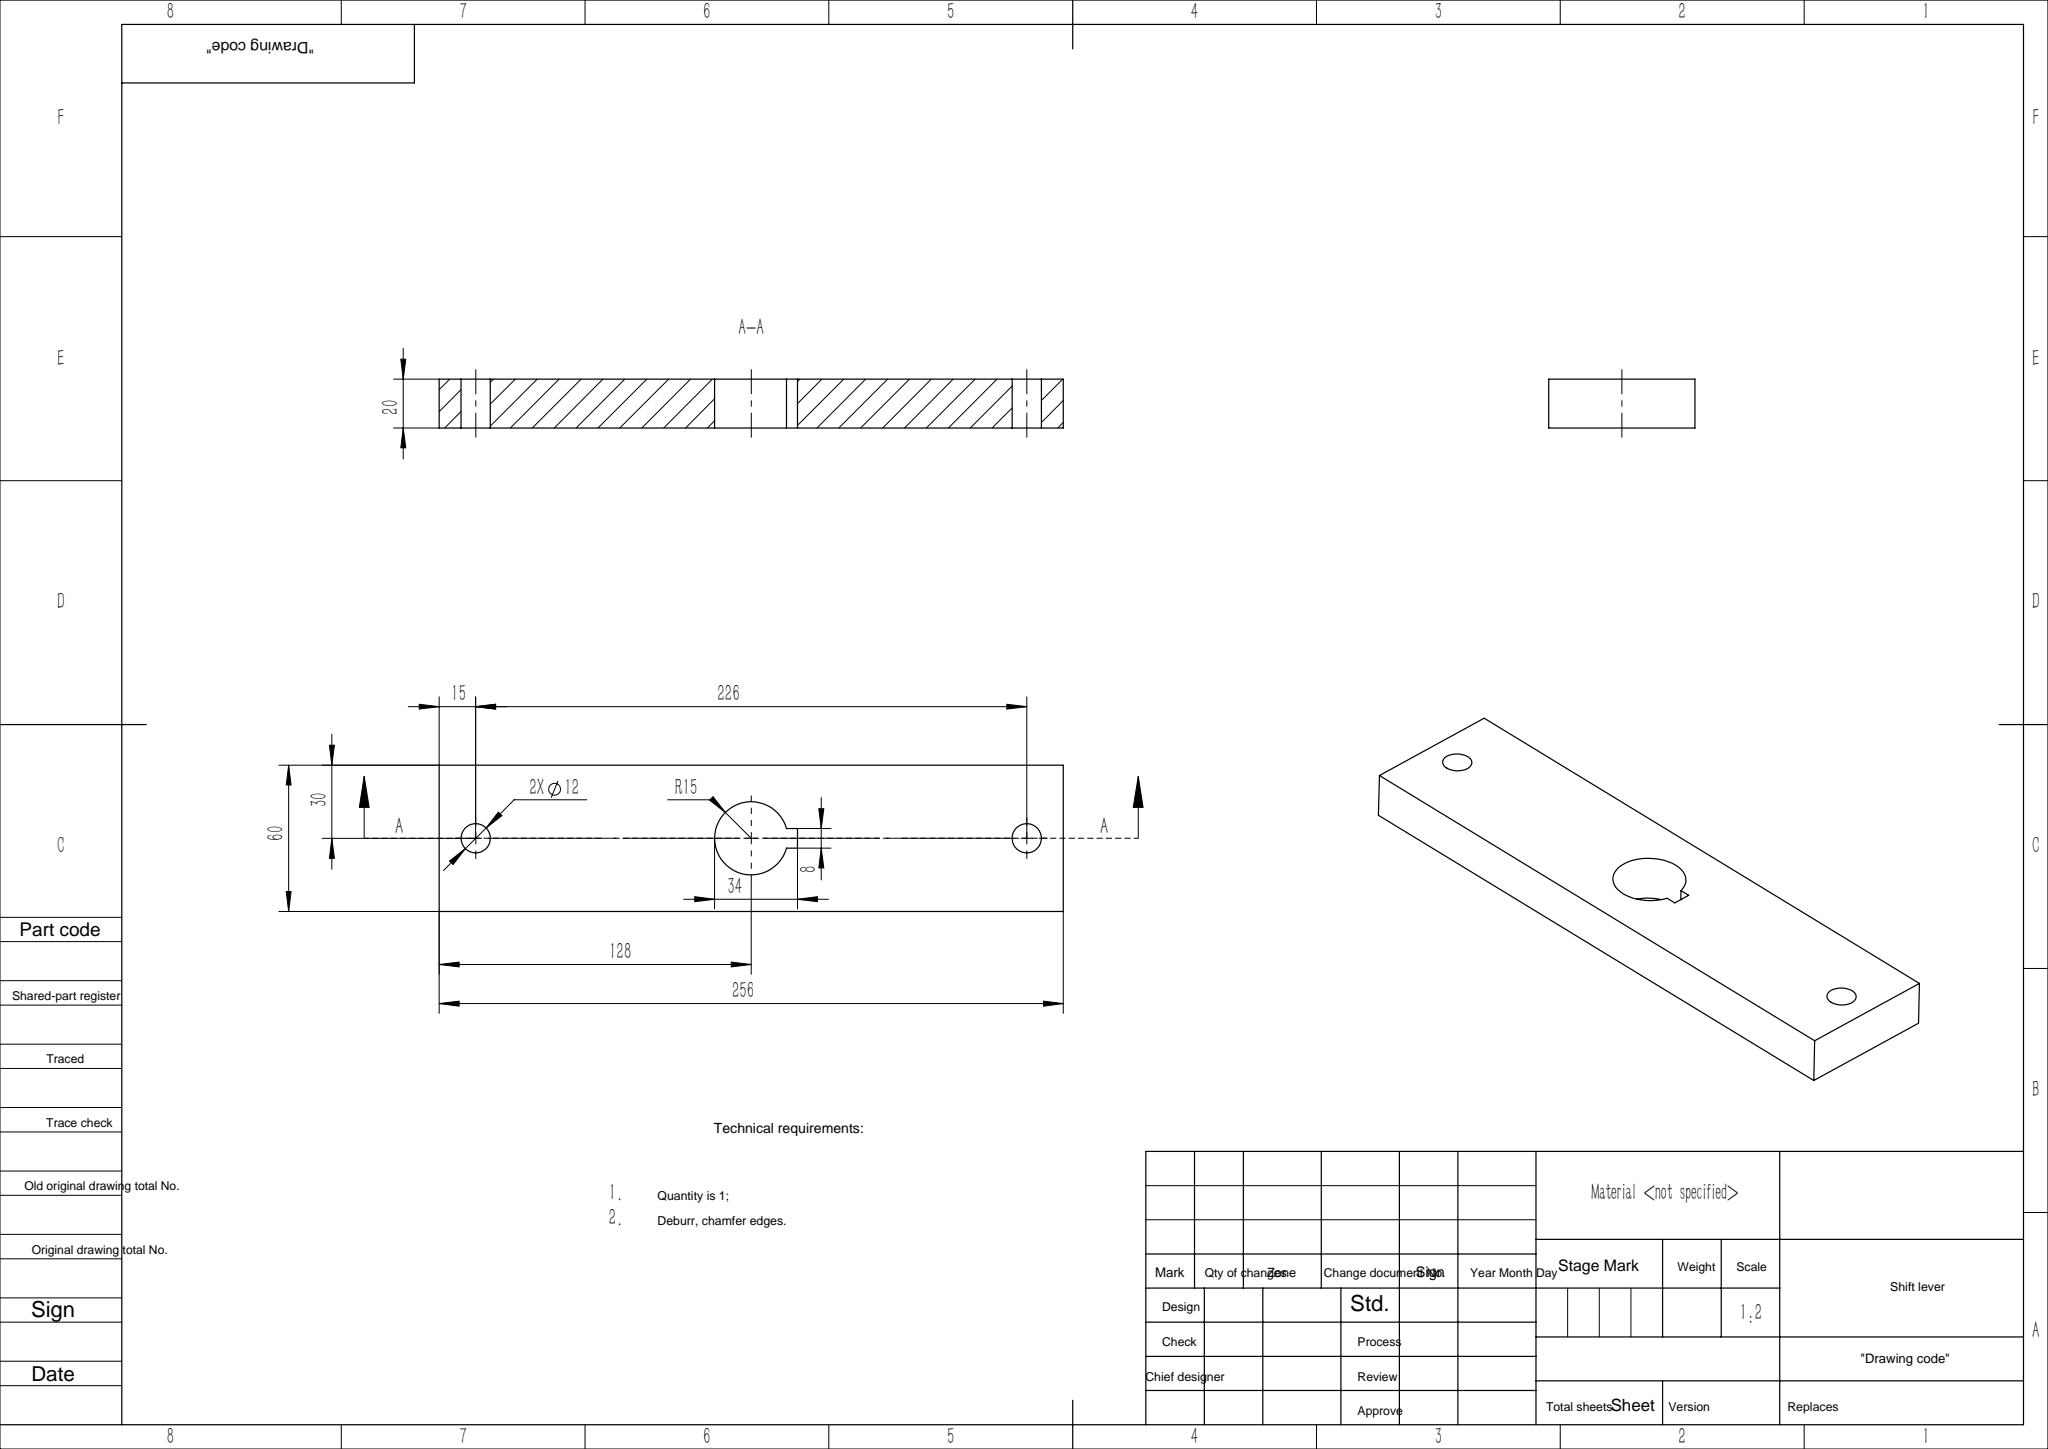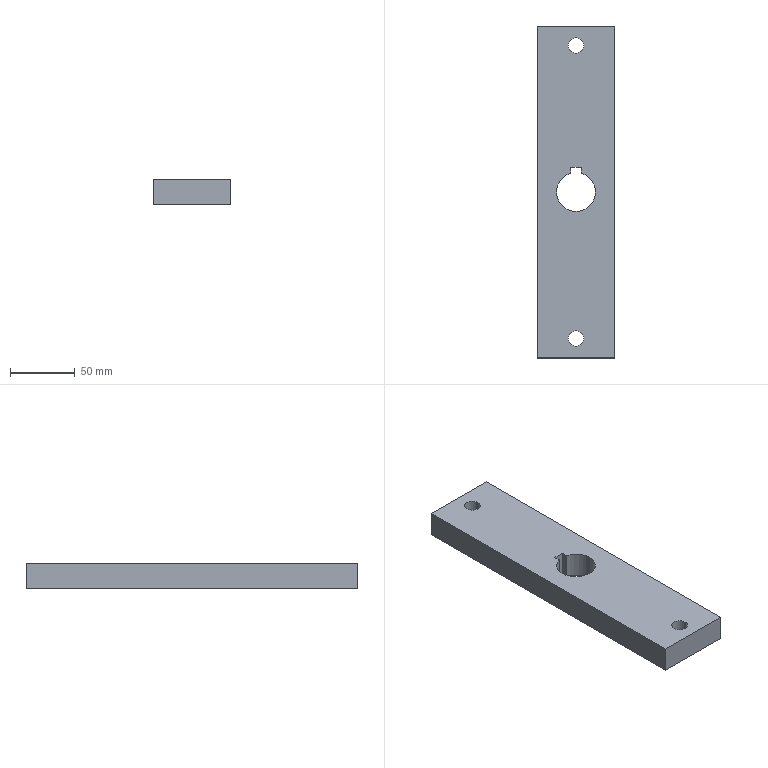Part | SolidWorks | features ICE 2, Extrusion 1 | 1 solid | 16 faces | box 60 x 256 x 20 mm | volume 287870 mm3 | plane 9 | cylinder 7 | commonest cylinder face diameters 12 x4 30 x3
STEP:
#1=CARTESIAN_POINT('',(-15.,0.,0.));
#2=VERTEX_POINT('',#1);
#3=CARTESIAN_POINT('',(15.,0.,0.));
#4=VERTEX_POINT('',#3);
#5=CARTESIAN_POINT('',(0.,0.,0.));
#6=DIRECTION('',(0.,0.,1.));
#7=DIRECTION('',(1.,0.,0.));
#8=AXIS2_PLACEMENT_3D('',#5,#6,#7);
#9=CIRCLE('',#8,15.);
#10=EDGE_CURVE('',#2,#4,#9,.T.);
#11=ORIENTED_EDGE('',*,*,#10,.F.);
#12=CARTESIAN_POINT('',(-15.,0.,20.));
#13=VERTEX_POINT('',#12);
#14=CARTESIAN_POINT('',(-15.,0.,0.));
#15=DIRECTION('',(0.,0.,1.));
#16=VECTOR('',#15,1000.);
#17=LINE('',#14,#16);
#18=EDGE_CURVE('',#2,#13,#17,.T.);
#19=ORIENTED_EDGE('',*,*,#18,.T.);
#20=CARTESIAN_POINT('',(15.,0.,20.));
#21=VERTEX_POINT('',#20);
#22=CARTESIAN_POINT('',(0.,0.,20.));
#23=DIRECTION('',(0.,0.,1.));
#24=DIRECTION('',(1.,0.,0.));
#25=AXIS2_PLACEMENT_3D('',#22,#23,#24);
#26=CIRCLE('',#25,15.);
#27=EDGE_CURVE('',#13,#21,#26,.T.);
#28=ORIENTED_EDGE('',*,*,#27,.T.);
#29=CARTESIAN_POINT('',(15.,0.,0.));
#30=DIRECTION('',(0.,0.,1.));
#31=VECTOR('',#30,1000.);
#32=LINE('',#29,#31);
#33=EDGE_CURVE('',#4,#21,#32,.T.);
#34=ORIENTED_EDGE('',*,*,#33,.F.);
#35=EDGE_LOOP('',(#11,#19,#28,#34));
#36=FACE_OUTER_BOUND('',#35,.T.);
#37=CARTESIAN_POINT('',(0.,0.,0.));
#38=DIRECTION('',(0.,0.,1.));
#39=DIRECTION('',(1.,0.,0.));
#40=AXIS2_PLACEMENT_3D('',#37,#38,#39);
#41=CYLINDRICAL_SURFACE('',#40,15.);
#42=ADVANCED_FACE('',(#36),#41,.F.);
#43=CARTESIAN_POINT('',(4.,14.457,0.));
#44=VERTEX_POINT('',#43);
#45=CARTESIAN_POINT('',(0.,0.,0.));
#46=DIRECTION('',(0.,0.,1.));
#47=DIRECTION('',(1.,0.,0.));
#48=AXIS2_PLACEMENT_3D('',#45,#46,#47);
#49=CIRCLE('',#48,15.);
#50=EDGE_CURVE('',#4,#44,#49,.T.);
#51=ORIENTED_EDGE('',*,*,#50,.F.);
#52=ORIENTED_EDGE('',*,*,#33,.T.);
#53=CARTESIAN_POINT('',(4.,14.457,20.));
#54=VERTEX_POINT('',#53);
#55=CARTESIAN_POINT('',(0.,0.,20.));
#56=DIRECTION('',(0.,0.,1.));
#57=DIRECTION('',(1.,0.,0.));
#58=AXIS2_PLACEMENT_3D('',#55,#56,#57);
#59=CIRCLE('',#58,15.);
#60=EDGE_CURVE('',#21,#54,#59,.T.);
#61=ORIENTED_EDGE('',*,*,#60,.T.);
#62=CARTESIAN_POINT('',(4.,14.457,0.));
#63=DIRECTION('',(0.,0.,1.));
#64=VECTOR('',#63,1000.);
#65=LINE('',#62,#64);
#66=EDGE_CURVE('',#44,#54,#65,.T.);
#67=ORIENTED_EDGE('',*,*,#66,.F.);
#68=EDGE_LOOP('',(#51,#52,#61,#67));
#69=FACE_OUTER_BOUND('',#68,.T.);
#70=CARTESIAN_POINT('',(0.,0.,0.));
#71=DIRECTION('',(0.,0.,1.));
#72=DIRECTION('',(1.,0.,0.));
#73=AXIS2_PLACEMENT_3D('',#70,#71,#72);
#74=CYLINDRICAL_SURFACE('',#73,15.);
#75=ADVANCED_FACE('',(#69),#74,.F.);
#76=CARTESIAN_POINT('',(-6.,-113.,0.));
#77=VERTEX_POINT('',#76);
#78=CARTESIAN_POINT('',(6.,-113.,0.));
#79=VERTEX_POINT('',#78);
#80=CARTESIAN_POINT('',(0.,-113.,0.));
#81=DIRECTION('',(0.,0.,1.));
#82=DIRECTION('',(1.,0.,0.));
#83=AXIS2_PLACEMENT_3D('',#80,#81,#82);
#84=CIRCLE('',#83,6.);
#85=EDGE_CURVE('',#77,#79,#84,.T.);
#86=ORIENTED_EDGE('',*,*,#85,.F.);
#87=CARTESIAN_POINT('',(-6.,-113.,20.));
#88=VERTEX_POINT('',#87);
#89=CARTESIAN_POINT('',(-6.,-113.,0.));
#90=DIRECTION('',(0.,0.,1.));
#91=VECTOR('',#90,1000.);
#92=LINE('',#89,#91);
#93=EDGE_CURVE('',#77,#88,#92,.T.);
#94=ORIENTED_EDGE('',*,*,#93,.T.);
#95=CARTESIAN_POINT('',(6.,-113.,20.));
#96=VERTEX_POINT('',#95);
#97=CARTESIAN_POINT('',(0.,-113.,20.));
#98=DIRECTION('',(0.,0.,1.));
#99=DIRECTION('',(1.,0.,0.));
#100=AXIS2_PLACEMENT_3D('',#97,#98,#99);
#101=CIRCLE('',#100,6.);
#102=EDGE_CURVE('',#88,#96,#101,.T.);
#103=ORIENTED_EDGE('',*,*,#102,.T.);
#104=CARTESIAN_POINT('',(6.,-113.,0.));
#105=DIRECTION('',(0.,0.,1.));
#106=VECTOR('',#105,1000.);
#107=LINE('',#104,#106);
#108=EDGE_CURVE('',#79,#96,#107,.T.);
#109=ORIENTED_EDGE('',*,*,#108,.F.);
#110=EDGE_LOOP('',(#86,#94,#103,#109));
#111=FACE_OUTER_BOUND('',#110,.T.);
#112=CARTESIAN_POINT('',(0.,-113.,0.));
#113=DIRECTION('',(0.,0.,1.));
#114=DIRECTION('',(1.,0.,0.));
#115=AXIS2_PLACEMENT_3D('',#112,#113,#114);
#116=CYLINDRICAL_SURFACE('',#115,6.);
#117=ADVANCED_FACE('',(#111),#116,.F.);
#118=CARTESIAN_POINT('',(-6.,113.,0.));
#119=VERTEX_POINT('',#118);
#120=CARTESIAN_POINT('',(6.,113.,0.));
#121=VERTEX_POINT('',#120);
#122=CARTESIAN_POINT('',(0.,113.,0.));
#123=DIRECTION('',(0.,0.,1.));
#124=DIRECTION('',(1.,0.,0.));
#125=AXIS2_PLACEMENT_3D('',#122,#123,#124);
#126=CIRCLE('',#125,6.);
#127=EDGE_CURVE('',#119,#121,#126,.T.);
#128=ORIENTED_EDGE('',*,*,#127,.F.);
#129=CARTESIAN_POINT('',(-6.,113.,20.));
#130=VERTEX_POINT('',#129);
#131=CARTESIAN_POINT('',(-6.,113.,0.));
#132=DIRECTION('',(0.,0.,1.));
#133=VECTOR('',#132,1000.);
#134=LINE('',#131,#133);
#135=EDGE_CURVE('',#119,#130,#134,.T.);
#136=ORIENTED_EDGE('',*,*,#135,.T.);
#137=CARTESIAN_POINT('',(6.,113.,20.));
#138=VERTEX_POINT('',#137);
#139=CARTESIAN_POINT('',(0.,113.,20.));
#140=DIRECTION('',(0.,0.,1.));
#141=DIRECTION('',(1.,0.,0.));
#142=AXIS2_PLACEMENT_3D('',#139,#140,#141);
#143=CIRCLE('',#142,6.);
#144=EDGE_CURVE('',#130,#138,#143,.T.);
#145=ORIENTED_EDGE('',*,*,#144,.T.);
#146=CARTESIAN_POINT('',(6.,113.,0.));
#147=DIRECTION('',(0.,0.,1.));
#148=VECTOR('',#147,1000.);
#149=LINE('',#146,#148);
#150=EDGE_CURVE('',#121,#138,#149,.T.);
#151=ORIENTED_EDGE('',*,*,#150,.F.);
#152=EDGE_LOOP('',(#128,#136,#145,#151));
#153=FACE_OUTER_BOUND('',#152,.T.);
#154=CARTESIAN_POINT('',(0.,113.,0.));
#155=DIRECTION('',(0.,0.,1.));
#156=DIRECTION('',(1.,0.,0.));
#157=AXIS2_PLACEMENT_3D('',#154,#155,#156);
#158=CYLINDRICAL_SURFACE('',#157,6.);
#159=ADVANCED_FACE('',(#153),#158,.F.);
#160=CARTESIAN_POINT('',(30.,-128.,0.));
#161=VERTEX_POINT('',#160);
#162=CARTESIAN_POINT('',(30.,128.,0.));
#163=VERTEX_POINT('',#162);
#164=CARTESIAN_POINT('',(30.,-128.,0.));
#165=DIRECTION('',(0.,1.,0.));
#166=VECTOR('',#165,1000.);
#167=LINE('',#164,#166);
#168=EDGE_CURVE('',#161,#163,#167,.T.);
#169=ORIENTED_EDGE('',*,*,#168,.T.);
#170=CARTESIAN_POINT('',(30.,128.,20.));
#171=VERTEX_POINT('',#170);
#172=CARTESIAN_POINT('',(30.,128.,20.));
#173=DIRECTION('',(0.,0.,-1.));
#174=VECTOR('',#173,1000.);
#175=LINE('',#172,#174);
#176=EDGE_CURVE('',#171,#163,#175,.T.);
#177=ORIENTED_EDGE('',*,*,#176,.F.);
#178=CARTESIAN_POINT('',(30.,-128.,20.));
#179=VERTEX_POINT('',#178);
#180=CARTESIAN_POINT('',(30.,-128.,20.));
#181=DIRECTION('',(0.,1.,0.));
#182=VECTOR('',#181,1000.);
#183=LINE('',#180,#182);
#184=EDGE_CURVE('',#179,#171,#183,.T.);
#185=ORIENTED_EDGE('',*,*,#184,.F.);
#186=CARTESIAN_POINT('',(30.,-128.,20.));
#187=DIRECTION('',(0.,0.,-1.));
#188=VECTOR('',#187,1000.);
#189=LINE('',#186,#188);
#190=EDGE_CURVE('',#179,#161,#189,.T.);
#191=ORIENTED_EDGE('',*,*,#190,.T.);
#192=EDGE_LOOP('',(#169,#177,#185,#191));
#193=FACE_OUTER_BOUND('',#192,.T.);
#194=CARTESIAN_POINT('',(30.,-128.,20.));
#195=DIRECTION('',(-1.,0.,0.));
#196=DIRECTION('',(0.,0.,1.));
#197=AXIS2_PLACEMENT_3D('',#194,#195,#196);
#198=PLANE('',#197);
#199=ADVANCED_FACE('',(#193),#198,.F.);
#200=CARTESIAN_POINT('',(-30.,128.,0.));
#201=VERTEX_POINT('',#200);
#202=CARTESIAN_POINT('',(-30.,128.,0.));
#203=DIRECTION('',(-1.,0.,0.));
#204=VECTOR('',#203,1000.);
#205=LINE('',#202,#204);
#206=EDGE_CURVE('',#163,#201,#205,.T.);
#207=ORIENTED_EDGE('',*,*,#206,.T.);
#208=CARTESIAN_POINT('',(-30.,128.,20.));
#209=VERTEX_POINT('',#208);
#210=CARTESIAN_POINT('',(-30.,128.,20.));
#211=DIRECTION('',(0.,0.,-1.));
#212=VECTOR('',#211,1000.);
#213=LINE('',#210,#212);
#214=EDGE_CURVE('',#209,#201,#213,.T.);
#215=ORIENTED_EDGE('',*,*,#214,.F.);
#216=CARTESIAN_POINT('',(-30.,128.,20.));
#217=DIRECTION('',(-1.,0.,0.));
#218=VECTOR('',#217,1000.);
#219=LINE('',#216,#218);
#220=EDGE_CURVE('',#171,#209,#219,.T.);
#221=ORIENTED_EDGE('',*,*,#220,.F.);
#222=ORIENTED_EDGE('',*,*,#176,.T.);
#223=EDGE_LOOP('',(#207,#215,#221,#222));
#224=FACE_OUTER_BOUND('',#223,.T.);
#225=CARTESIAN_POINT('',(-30.,128.,20.));
#226=DIRECTION('',(0.,-1.,0.));
#227=DIRECTION('',(0.,0.,-1.));
#228=AXIS2_PLACEMENT_3D('',#225,#226,#227);
#229=PLANE('',#228);
#230=ADVANCED_FACE('',(#224),#229,.F.);
#231=CARTESIAN_POINT('',(-30.,-128.,0.));
#232=VERTEX_POINT('',#231);
#233=CARTESIAN_POINT('',(-30.,-128.,0.));
#234=DIRECTION('',(0.,-1.,0.));
#235=VECTOR('',#234,1000.);
#236=LINE('',#233,#235);
#237=EDGE_CURVE('',#201,#232,#236,.T.);
#238=ORIENTED_EDGE('',*,*,#237,.T.);
#239=CARTESIAN_POINT('',(-30.,-128.,20.));
#240=VERTEX_POINT('',#239);
#241=CARTESIAN_POINT('',(-30.,-128.,20.));
#242=DIRECTION('',(0.,0.,-1.));
#243=VECTOR('',#242,1000.);
#244=LINE('',#241,#243);
#245=EDGE_CURVE('',#240,#232,#244,.T.);
#246=ORIENTED_EDGE('',*,*,#245,.F.);
#247=CARTESIAN_POINT('',(-30.,-128.,20.));
#248=DIRECTION('',(0.,-1.,0.));
#249=VECTOR('',#248,1000.);
#250=LINE('',#247,#249);
#251=EDGE_CURVE('',#209,#240,#250,.T.);
#252=ORIENTED_EDGE('',*,*,#251,.F.);
#253=ORIENTED_EDGE('',*,*,#214,.T.);
#254=EDGE_LOOP('',(#238,#246,#252,#253));
#255=FACE_OUTER_BOUND('',#254,.T.);
#256=CARTESIAN_POINT('',(-30.,-128.,20.));
#257=DIRECTION('',(1.,0.,0.));
#258=DIRECTION('',(0.,0.,-1.));
#259=AXIS2_PLACEMENT_3D('',#256,#257,#258);
#260=PLANE('',#259);
#261=ADVANCED_FACE('',(#255),#260,.F.);
#262=CARTESIAN_POINT('',(-30.,-128.,0.));
#263=DIRECTION('',(1.,0.,0.));
#264=VECTOR('',#263,1000.);
#265=LINE('',#262,#264);
#266=EDGE_CURVE('',#232,#161,#265,.T.);
#267=ORIENTED_EDGE('',*,*,#266,.T.);
#268=ORIENTED_EDGE('',*,*,#190,.F.);
#269=CARTESIAN_POINT('',(-30.,-128.,20.));
#270=DIRECTION('',(1.,0.,0.));
#271=VECTOR('',#270,1000.);
#272=LINE('',#269,#271);
#273=EDGE_CURVE('',#240,#179,#272,.T.);
#274=ORIENTED_EDGE('',*,*,#273,.F.);
#275=ORIENTED_EDGE('',*,*,#245,.T.);
#276=EDGE_LOOP('',(#267,#268,#274,#275));
#277=FACE_OUTER_BOUND('',#276,.T.);
#278=CARTESIAN_POINT('',(-30.,-128.,20.));
#279=DIRECTION('',(0.,1.,0.));
#280=DIRECTION('',(0.,0.,1.));
#281=AXIS2_PLACEMENT_3D('',#278,#279,#280);
#282=PLANE('',#281);
#283=ADVANCED_FACE('',(#277),#282,.F.);
#284=CARTESIAN_POINT('',(-4.,14.457,20.));
#285=VERTEX_POINT('',#284);
#286=CARTESIAN_POINT('',(0.,0.,20.));
#287=DIRECTION('',(0.,0.,1.));
#288=DIRECTION('',(1.,0.,0.));
#289=AXIS2_PLACEMENT_3D('',#286,#287,#288);
#290=CIRCLE('',#289,15.);
#291=EDGE_CURVE('',#285,#13,#290,.T.);
#292=ORIENTED_EDGE('',*,*,#291,.F.);
#293=CARTESIAN_POINT('',(-4.,19.,20.));
#294=VERTEX_POINT('',#293);
#295=CARTESIAN_POINT('',(-4.,19.,20.));
#296=DIRECTION('',(0.,-1.,0.));
#297=VECTOR('',#296,1000.);
#298=LINE('',#295,#297);
#299=EDGE_CURVE('',#294,#285,#298,.T.);
#300=ORIENTED_EDGE('',*,*,#299,.F.);
#301=CARTESIAN_POINT('',(4.,19.,20.));
#302=VERTEX_POINT('',#301);
#303=CARTESIAN_POINT('',(-4.,19.,20.));
#304=DIRECTION('',(-1.,0.,0.));
#305=VECTOR('',#304,1000.);
#306=LINE('',#303,#305);
#307=EDGE_CURVE('',#302,#294,#306,.T.);
#308=ORIENTED_EDGE('',*,*,#307,.F.);
#309=CARTESIAN_POINT('',(4.,19.,20.));
#310=DIRECTION('',(0.,1.,0.));
#311=VECTOR('',#310,1000.);
#312=LINE('',#309,#311);
#313=EDGE_CURVE('',#54,#302,#312,.T.);
#314=ORIENTED_EDGE('',*,*,#313,.F.);
#315=ORIENTED_EDGE('',*,*,#60,.F.);
#316=ORIENTED_EDGE('',*,*,#27,.F.);
#317=EDGE_LOOP('',(#292,#300,#308,#314,#315,#316));
#318=FACE_BOUND('',#317,.T.);
#319=CARTESIAN_POINT('',(0.,-113.,20.));
#320=DIRECTION('',(0.,0.,1.));
#321=DIRECTION('',(1.,0.,0.));
#322=AXIS2_PLACEMENT_3D('',#319,#320,#321);
#323=CIRCLE('',#322,6.);
#324=EDGE_CURVE('',#96,#88,#323,.T.);
#325=ORIENTED_EDGE('',*,*,#324,.F.);
#326=ORIENTED_EDGE('',*,*,#102,.F.);
#327=EDGE_LOOP('',(#325,#326));
#328=FACE_BOUND('',#327,.T.);
#329=CARTESIAN_POINT('',(0.,113.,20.));
#330=DIRECTION('',(0.,0.,1.));
#331=DIRECTION('',(1.,0.,0.));
#332=AXIS2_PLACEMENT_3D('',#329,#330,#331);
#333=CIRCLE('',#332,6.);
#334=EDGE_CURVE('',#138,#130,#333,.T.);
#335=ORIENTED_EDGE('',*,*,#334,.F.);
#336=ORIENTED_EDGE('',*,*,#144,.F.);
#337=EDGE_LOOP('',(#335,#336));
#338=FACE_BOUND('',#337,.T.);
#339=ORIENTED_EDGE('',*,*,#184,.T.);
#340=ORIENTED_EDGE('',*,*,#220,.T.);
#341=ORIENTED_EDGE('',*,*,#251,.T.);
#342=ORIENTED_EDGE('',*,*,#273,.T.);
#343=EDGE_LOOP('',(#339,#340,#341,#342));
#344=FACE_OUTER_BOUND('',#343,.T.);
#345=CARTESIAN_POINT('',(0.,0.,20.));
#346=DIRECTION('',(0.,0.,-1.));
#347=DIRECTION('',(-1.,0.,0.));
#348=AXIS2_PLACEMENT_3D('',#345,#346,#347);
#349=PLANE('',#348);
#350=ADVANCED_FACE('',(#318,#328,#338,#344),#349,.F.);
#351=CARTESIAN_POINT('',(-4.,19.,0.));
#352=VERTEX_POINT('',#351);
#353=CARTESIAN_POINT('',(-4.,14.457,0.));
#354=VERTEX_POINT('',#353);
#355=CARTESIAN_POINT('',(-4.,19.,0.));
#356=DIRECTION('',(0.,-1.,0.));
#357=VECTOR('',#356,1000.);
#358=LINE('',#355,#357);
#359=EDGE_CURVE('',#352,#354,#358,.T.);
#360=ORIENTED_EDGE('',*,*,#359,.T.);
#361=CARTESIAN_POINT('',(0.,0.,0.));
#362=DIRECTION('',(0.,0.,1.));
#363=DIRECTION('',(1.,0.,0.));
#364=AXIS2_PLACEMENT_3D('',#361,#362,#363);
#365=CIRCLE('',#364,15.);
#366=EDGE_CURVE('',#354,#2,#365,.T.);
#367=ORIENTED_EDGE('',*,*,#366,.T.);
#368=ORIENTED_EDGE('',*,*,#10,.T.);
#369=ORIENTED_EDGE('',*,*,#50,.T.);
#370=CARTESIAN_POINT('',(4.,19.,0.));
#371=VERTEX_POINT('',#370);
#372=CARTESIAN_POINT('',(4.,19.,0.));
#373=DIRECTION('',(0.,1.,0.));
#374=VECTOR('',#373,1000.);
#375=LINE('',#372,#374);
#376=EDGE_CURVE('',#44,#371,#375,.T.);
#377=ORIENTED_EDGE('',*,*,#376,.T.);
#378=CARTESIAN_POINT('',(-4.,19.,0.));
#379=DIRECTION('',(-1.,0.,0.));
#380=VECTOR('',#379,1000.);
#381=LINE('',#378,#380);
#382=EDGE_CURVE('',#371,#352,#381,.T.);
#383=ORIENTED_EDGE('',*,*,#382,.T.);
#384=EDGE_LOOP('',(#360,#367,#368,#369,#377,#383));
#385=FACE_BOUND('',#384,.T.);
#386=CARTESIAN_POINT('',(0.,-113.,0.));
#387=DIRECTION('',(0.,0.,1.));
#388=DIRECTION('',(1.,0.,0.));
#389=AXIS2_PLACEMENT_3D('',#386,#387,#388);
#390=CIRCLE('',#389,6.);
#391=EDGE_CURVE('',#79,#77,#390,.T.);
#392=ORIENTED_EDGE('',*,*,#391,.T.);
#393=ORIENTED_EDGE('',*,*,#85,.T.);
#394=EDGE_LOOP('',(#392,#393));
#395=FACE_BOUND('',#394,.T.);
#396=CARTESIAN_POINT('',(0.,113.,0.));
#397=DIRECTION('',(0.,0.,1.));
#398=DIRECTION('',(1.,0.,0.));
#399=AXIS2_PLACEMENT_3D('',#396,#397,#398);
#400=CIRCLE('',#399,6.);
#401=EDGE_CURVE('',#121,#119,#400,.T.);
#402=ORIENTED_EDGE('',*,*,#401,.T.);
#403=ORIENTED_EDGE('',*,*,#127,.T.);
#404=EDGE_LOOP('',(#402,#403));
#405=FACE_BOUND('',#404,.T.);
#406=ORIENTED_EDGE('',*,*,#168,.F.);
#407=ORIENTED_EDGE('',*,*,#266,.F.);
#408=ORIENTED_EDGE('',*,*,#237,.F.);
#409=ORIENTED_EDGE('',*,*,#206,.F.);
#410=EDGE_LOOP('',(#406,#407,#408,#409));
#411=FACE_OUTER_BOUND('',#410,.T.);
#412=CARTESIAN_POINT('',(0.,0.,0.));
#413=DIRECTION('',(0.,0.,-1.));
#414=DIRECTION('',(-1.,0.,0.));
#415=AXIS2_PLACEMENT_3D('',#412,#413,#414);
#416=PLANE('',#415);
#417=ADVANCED_FACE('',(#385,#395,#405,#411),#416,.T.);
#418=ORIENTED_EDGE('',*,*,#135,.F.);
#419=ORIENTED_EDGE('',*,*,#401,.F.);
#420=ORIENTED_EDGE('',*,*,#150,.T.);
#421=ORIENTED_EDGE('',*,*,#334,.T.);
#422=EDGE_LOOP('',(#418,#419,#420,#421));
#423=FACE_OUTER_BOUND('',#422,.T.);
#424=CARTESIAN_POINT('',(0.,113.,0.));
#425=DIRECTION('',(0.,0.,1.));
#426=DIRECTION('',(1.,0.,0.));
#427=AXIS2_PLACEMENT_3D('',#424,#425,#426);
#428=CYLINDRICAL_SURFACE('',#427,6.);
#429=ADVANCED_FACE('',(#423),#428,.F.);
#430=ORIENTED_EDGE('',*,*,#93,.F.);
#431=ORIENTED_EDGE('',*,*,#391,.F.);
#432=ORIENTED_EDGE('',*,*,#108,.T.);
#433=ORIENTED_EDGE('',*,*,#324,.T.);
#434=EDGE_LOOP('',(#430,#431,#432,#433));
#435=FACE_OUTER_BOUND('',#434,.T.);
#436=CARTESIAN_POINT('',(0.,-113.,0.));
#437=DIRECTION('',(0.,0.,1.));
#438=DIRECTION('',(1.,0.,0.));
#439=AXIS2_PLACEMENT_3D('',#436,#437,#438);
#440=CYLINDRICAL_SURFACE('',#439,6.);
#441=ADVANCED_FACE('',(#435),#440,.F.);
#442=ORIENTED_EDGE('',*,*,#299,.T.);
#443=CARTESIAN_POINT('',(-4.,14.457,0.));
#444=DIRECTION('',(0.,0.,1.));
#445=VECTOR('',#444,1000.);
#446=LINE('',#443,#445);
#447=EDGE_CURVE('',#354,#285,#446,.T.);
#448=ORIENTED_EDGE('',*,*,#447,.F.);
#449=ORIENTED_EDGE('',*,*,#359,.F.);
#450=CARTESIAN_POINT('',(-4.,19.,0.));
#451=DIRECTION('',(0.,0.,1.));
#452=VECTOR('',#451,1000.);
#453=LINE('',#450,#452);
#454=EDGE_CURVE('',#352,#294,#453,.T.);
#455=ORIENTED_EDGE('',*,*,#454,.T.);
#456=EDGE_LOOP('',(#442,#448,#449,#455));
#457=FACE_OUTER_BOUND('',#456,.T.);
#458=CARTESIAN_POINT('',(-4.,19.,0.));
#459=DIRECTION('',(-1.,0.,0.));
#460=DIRECTION('',(0.,-1.,0.));
#461=AXIS2_PLACEMENT_3D('',#458,#459,#460);
#462=PLANE('',#461);
#463=ADVANCED_FACE('',(#457),#462,.F.);
#464=ORIENTED_EDGE('',*,*,#307,.T.);
#465=ORIENTED_EDGE('',*,*,#454,.F.);
#466=ORIENTED_EDGE('',*,*,#382,.F.);
#467=CARTESIAN_POINT('',(4.,19.,0.));
#468=DIRECTION('',(0.,0.,1.));
#469=VECTOR('',#468,1000.);
#470=LINE('',#467,#469);
#471=EDGE_CURVE('',#371,#302,#470,.T.);
#472=ORIENTED_EDGE('',*,*,#471,.T.);
#473=EDGE_LOOP('',(#464,#465,#466,#472));
#474=FACE_OUTER_BOUND('',#473,.T.);
#475=CARTESIAN_POINT('',(-4.,19.,0.));
#476=DIRECTION('',(0.,1.,0.));
#477=DIRECTION('',(0.,0.,1.));
#478=AXIS2_PLACEMENT_3D('',#475,#476,#477);
#479=PLANE('',#478);
#480=ADVANCED_FACE('',(#474),#479,.F.);
#481=ORIENTED_EDGE('',*,*,#313,.T.);
#482=ORIENTED_EDGE('',*,*,#471,.F.);
#483=ORIENTED_EDGE('',*,*,#376,.F.);
#484=ORIENTED_EDGE('',*,*,#66,.T.);
#485=EDGE_LOOP('',(#481,#482,#483,#484));
#486=FACE_OUTER_BOUND('',#485,.T.);
#487=CARTESIAN_POINT('',(4.,19.,0.));
#488=DIRECTION('',(1.,0.,0.));
#489=DIRECTION('',(0.,1.,0.));
#490=AXIS2_PLACEMENT_3D('',#487,#488,#489);
#491=PLANE('',#490);
#492=ADVANCED_FACE('',(#486),#491,.F.);
#493=ORIENTED_EDGE('',*,*,#18,.F.);
#494=ORIENTED_EDGE('',*,*,#366,.F.);
#495=ORIENTED_EDGE('',*,*,#447,.T.);
#496=ORIENTED_EDGE('',*,*,#291,.T.);
#497=EDGE_LOOP('',(#493,#494,#495,#496));
#498=FACE_OUTER_BOUND('',#497,.T.);
#499=CARTESIAN_POINT('',(0.,0.,0.));
#500=DIRECTION('',(0.,0.,1.));
#501=DIRECTION('',(1.,0.,0.));
#502=AXIS2_PLACEMENT_3D('',#499,#500,#501);
#503=CYLINDRICAL_SURFACE('',#502,15.);
#504=ADVANCED_FACE('',(#498),#503,.F.);
#505=CLOSED_SHELL('',(#42,#75,#117,#159,#199,#230,#261,#283,#350,#417,#429,#441,#463,#480,#492,#504));
#506=MANIFOLD_SOLID_BREP('',#505);
#507=CARTESIAN_POINT('',(0.,0.,0.));
#508=DIRECTION('',(0.,0.,1.));
#509=DIRECTION('',(1.,0.,0.));
#510=AXIS2_PLACEMENT_3D('',#507,#508,#509);
#511=(LENGTH_UNIT()NAMED_UNIT(*)SI_UNIT(.MILLI.,.METRE.));
#512=UNCERTAINTY_MEASURE_WITH_UNIT(LENGTH_MEASURE(0.00001),#511,'','');
#513=(NAMED_UNIT(*)PLANE_ANGLE_UNIT()SI_UNIT($,.RADIAN.));
#514=(NAMED_UNIT(*)SI_UNIT($,.STERADIAN.)SOLID_ANGLE_UNIT());
#515=(GEOMETRIC_REPRESENTATION_CONTEXT(3)GLOBAL_UNCERTAINTY_ASSIGNED_CONTEXT((#512))GLOBAL_UNIT_ASSIGNED_CONTEXT((#511,#513,#514))REPRESENTATION_CONTEXT('',''));
#516=ADVANCED_BREP_SHAPE_REPRESENTATION('',(#506,#510),#515);